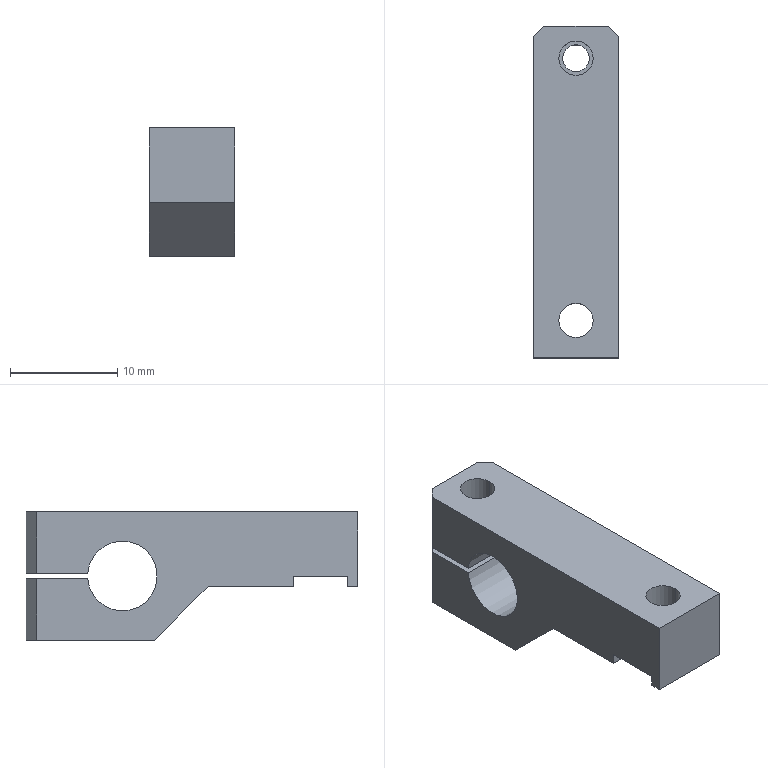Part | SolidWorks | features ICE 4, HoleWzd 3, Chamfer 2, Extrusion 1 | 1 solid | 26 faces | box 8 x 31 x 12 mm | volume 1853 mm3 | plane 19 | cylinder 7 | commonest cylinder face diameters 3.2 x4 2.5 x2 6.5 x1
STEP:
#1=CARTESIAN_POINT('',(-1.6,-12.,0.));
#2=VERTEX_POINT('',#1);
#3=CARTESIAN_POINT('',(1.6,-12.,0.));
#4=VERTEX_POINT('',#3);
#5=CARTESIAN_POINT('',(0.,-12.,0.));
#6=DIRECTION('',(0.,0.,1.));
#7=DIRECTION('',(1.,0.,0.));
#8=AXIS2_PLACEMENT_3D('',#5,#6,#7);
#9=CIRCLE('',#8,1.6);
#10=EDGE_CURVE('',#2,#4,#9,.T.);
#11=ORIENTED_EDGE('',*,*,#10,.F.);
#12=CARTESIAN_POINT('',(-1.6,-12.,6.));
#13=VERTEX_POINT('',#12);
#14=CARTESIAN_POINT('',(-1.6,-12.,6.));
#15=DIRECTION('',(0.,0.,1.));
#16=VECTOR('',#15,1000.);
#17=LINE('',#14,#16);
#18=EDGE_CURVE('',#2,#13,#17,.T.);
#19=ORIENTED_EDGE('',*,*,#18,.T.);
#20=CARTESIAN_POINT('',(1.6,-12.,6.));
#21=VERTEX_POINT('',#20);
#22=CARTESIAN_POINT('',(0.,-12.,6.));
#23=DIRECTION('',(0.,0.,1.));
#24=DIRECTION('',(1.,0.,0.));
#25=AXIS2_PLACEMENT_3D('',#22,#23,#24);
#26=CIRCLE('',#25,1.6);
#27=EDGE_CURVE('',#13,#21,#26,.T.);
#28=ORIENTED_EDGE('',*,*,#27,.T.);
#29=CARTESIAN_POINT('',(1.6,-12.,6.));
#30=DIRECTION('',(0.,0.,1.));
#31=VECTOR('',#30,1000.);
#32=LINE('',#29,#31);
#33=EDGE_CURVE('',#4,#21,#32,.T.);
#34=ORIENTED_EDGE('',*,*,#33,.F.);
#35=EDGE_LOOP('',(#11,#19,#28,#34));
#36=FACE_OUTER_BOUND('',#35,.T.);
#37=CARTESIAN_POINT('',(0.,-12.,6.));
#38=DIRECTION('',(0.,0.,1.));
#39=DIRECTION('',(1.,0.,0.));
#40=AXIS2_PLACEMENT_3D('',#37,#38,#39);
#41=CYLINDRICAL_SURFACE('',#40,1.6);
#42=ADVANCED_FACE('',(#36),#41,.F.);
#43=CARTESIAN_POINT('',(1.6,12.5,0.25));
#44=VERTEX_POINT('',#43);
#45=CARTESIAN_POINT('',(-1.6,12.5,0.25));
#46=VERTEX_POINT('',#45);
#47=CARTESIAN_POINT('',(0.,12.5,0.25));
#48=DIRECTION('',(0.,0.,-1.));
#49=DIRECTION('',(0.,-1.,0.));
#50=AXIS2_PLACEMENT_3D('',#47,#48,#49);
#51=CIRCLE('',#50,1.6);
#52=EDGE_CURVE('',#44,#46,#51,.T.);
#53=ORIENTED_EDGE('',*,*,#52,.T.);
#54=CARTESIAN_POINT('',(-1.6,12.5,6.));
#55=VERTEX_POINT('',#54);
#56=CARTESIAN_POINT('',(-1.6,12.5,6.));
#57=DIRECTION('',(0.,0.,1.));
#58=VECTOR('',#57,1000.);
#59=LINE('',#56,#58);
#60=EDGE_CURVE('',#46,#55,#59,.T.);
#61=ORIENTED_EDGE('',*,*,#60,.T.);
#62=CARTESIAN_POINT('',(1.6,12.5,6.));
#63=VERTEX_POINT('',#62);
#64=CARTESIAN_POINT('',(0.,12.5,6.));
#65=DIRECTION('',(0.,0.,1.));
#66=DIRECTION('',(1.,0.,0.));
#67=AXIS2_PLACEMENT_3D('',#64,#65,#66);
#68=CIRCLE('',#67,1.6);
#69=EDGE_CURVE('',#55,#63,#68,.T.);
#70=ORIENTED_EDGE('',*,*,#69,.T.);
#71=CARTESIAN_POINT('',(1.6,12.5,6.));
#72=DIRECTION('',(0.,0.,1.));
#73=VECTOR('',#72,1000.);
#74=LINE('',#71,#73);
#75=EDGE_CURVE('',#44,#63,#74,.T.);
#76=ORIENTED_EDGE('',*,*,#75,.F.);
#77=EDGE_LOOP('',(#53,#61,#70,#76));
#78=FACE_OUTER_BOUND('',#77,.T.);
#79=CARTESIAN_POINT('',(0.,12.5,6.));
#80=DIRECTION('',(0.,0.,1.));
#81=DIRECTION('',(1.,0.,0.));
#82=AXIS2_PLACEMENT_3D('',#79,#80,#81);
#83=CYLINDRICAL_SURFACE('',#82,1.6);
#84=ADVANCED_FACE('',(#78),#83,.F.);
#85=CARTESIAN_POINT('',(1.25,12.5,-0.25));
#86=VERTEX_POINT('',#85);
#87=CARTESIAN_POINT('',(-1.25,12.5,-0.25));
#88=VERTEX_POINT('',#87);
#89=CARTESIAN_POINT('',(0.,12.5,-0.25));
#90=DIRECTION('',(0.,0.,-1.));
#91=DIRECTION('',(0.,1.,0.));
#92=AXIS2_PLACEMENT_3D('',#89,#90,#91);
#93=CIRCLE('',#92,1.25);
#94=EDGE_CURVE('',#86,#88,#93,.T.);
#95=ORIENTED_EDGE('',*,*,#94,.F.);
#96=CARTESIAN_POINT('',(1.25,12.5,-6.));
#97=VERTEX_POINT('',#96);
#98=CARTESIAN_POINT('',(1.25,12.5,-6.));
#99=DIRECTION('',(0.,0.,-1.));
#100=VECTOR('',#99,1000.);
#101=LINE('',#98,#100);
#102=EDGE_CURVE('',#86,#97,#101,.T.);
#103=ORIENTED_EDGE('',*,*,#102,.T.);
#104=CARTESIAN_POINT('',(-1.25,12.5,-6.));
#105=VERTEX_POINT('',#104);
#106=CARTESIAN_POINT('',(0.,12.5,-6.));
#107=DIRECTION('',(0.,0.,-1.));
#108=DIRECTION('',(-1.,0.,0.));
#109=AXIS2_PLACEMENT_3D('',#106,#107,#108);
#110=CIRCLE('',#109,1.25);
#111=EDGE_CURVE('',#97,#105,#110,.T.);
#112=ORIENTED_EDGE('',*,*,#111,.T.);
#113=CARTESIAN_POINT('',(-1.25,12.5,-6.));
#114=DIRECTION('',(0.,0.,-1.));
#115=VECTOR('',#114,1000.);
#116=LINE('',#113,#115);
#117=EDGE_CURVE('',#88,#105,#116,.T.);
#118=ORIENTED_EDGE('',*,*,#117,.F.);
#119=EDGE_LOOP('',(#95,#103,#112,#118));
#120=FACE_OUTER_BOUND('',#119,.T.);
#121=CARTESIAN_POINT('',(0.,12.5,-6.));
#122=DIRECTION('',(0.,0.,-1.));
#123=DIRECTION('',(-1.,0.,0.));
#124=AXIS2_PLACEMENT_3D('',#121,#122,#123);
#125=CYLINDRICAL_SURFACE('',#124,1.25);
#126=ADVANCED_FACE('',(#120),#125,.F.);
#127=CARTESIAN_POINT('',(-3.,15.5,-0.25));
#128=VERTEX_POINT('',#127);
#129=CARTESIAN_POINT('',(3.,15.5,-0.25));
#130=VERTEX_POINT('',#129);
#131=CARTESIAN_POINT('',(-4.,15.5,-0.25));
#132=DIRECTION('',(1.,0.,0.));
#133=VECTOR('',#132,1000.);
#134=LINE('',#131,#133);
#135=EDGE_CURVE('',#128,#130,#134,.T.);
#136=ORIENTED_EDGE('',*,*,#135,.T.);
#137=CARTESIAN_POINT('',(3.,15.5,-6.));
#138=VERTEX_POINT('',#137);
#139=CARTESIAN_POINT('',(3.,15.5,6.));
#140=DIRECTION('',(0.,0.,-1.));
#141=VECTOR('',#140,1000.);
#142=LINE('',#139,#141);
#143=EDGE_CURVE('',#130,#138,#142,.T.);
#144=ORIENTED_EDGE('',*,*,#143,.T.);
#145=CARTESIAN_POINT('',(-3.,15.5,-6.));
#146=VERTEX_POINT('',#145);
#147=CARTESIAN_POINT('',(-4.,15.5,-6.));
#148=DIRECTION('',(-1.,0.,0.));
#149=VECTOR('',#148,1000.);
#150=LINE('',#147,#149);
#151=EDGE_CURVE('',#138,#146,#150,.T.);
#152=ORIENTED_EDGE('',*,*,#151,.T.);
#153=CARTESIAN_POINT('',(-3.,15.5,6.));
#154=DIRECTION('',(0.,0.,1.));
#155=VECTOR('',#154,1000.);
#156=LINE('',#153,#155);
#157=EDGE_CURVE('',#146,#128,#156,.T.);
#158=ORIENTED_EDGE('',*,*,#157,.T.);
#159=EDGE_LOOP('',(#136,#144,#152,#158));
#160=FACE_OUTER_BOUND('',#159,.T.);
#161=CARTESIAN_POINT('',(-4.,15.5,6.));
#162=DIRECTION('',(0.,-1.,0.));
#163=DIRECTION('',(0.,0.,-1.));
#164=AXIS2_PLACEMENT_3D('',#161,#162,#163);
#165=PLANE('',#164);
#166=ADVANCED_FACE('',(#160),#165,.F.);
#167=CARTESIAN_POINT('',(4.,-1.5,-1.));
#168=VERTEX_POINT('',#167);
#169=CARTESIAN_POINT('',(4.,-9.5,-1.));
#170=VERTEX_POINT('',#169);
#171=CARTESIAN_POINT('',(4.,-15.5,-1.));
#172=DIRECTION('',(0.,-1.,0.));
#173=VECTOR('',#172,1000.);
#174=LINE('',#171,#173);
#175=EDGE_CURVE('',#168,#170,#174,.T.);
#176=ORIENTED_EDGE('',*,*,#175,.T.);
#177=CARTESIAN_POINT('',(-4.,-9.5,-1.));
#178=VERTEX_POINT('',#177);
#179=CARTESIAN_POINT('',(-4.,-9.5,-1.));
#180=DIRECTION('',(1.,0.,0.));
#181=VECTOR('',#180,1000.);
#182=LINE('',#179,#181);
#183=EDGE_CURVE('',#178,#170,#182,.T.);
#184=ORIENTED_EDGE('',*,*,#183,.F.);
#185=CARTESIAN_POINT('',(-4.,-1.5,-1.));
#186=VERTEX_POINT('',#185);
#187=CARTESIAN_POINT('',(-4.,-15.5,-1.));
#188=DIRECTION('',(0.,-1.,0.));
#189=VECTOR('',#188,1000.);
#190=LINE('',#187,#189);
#191=EDGE_CURVE('',#186,#178,#190,.T.);
#192=ORIENTED_EDGE('',*,*,#191,.F.);
#193=CARTESIAN_POINT('',(-4.,-1.5,-1.));
#194=DIRECTION('',(1.,0.,0.));
#195=VECTOR('',#194,1000.);
#196=LINE('',#193,#195);
#197=EDGE_CURVE('',#186,#168,#196,.T.);
#198=ORIENTED_EDGE('',*,*,#197,.T.);
#199=EDGE_LOOP('',(#176,#184,#192,#198));
#200=FACE_OUTER_BOUND('',#199,.T.);
#201=CARTESIAN_POINT('',(-4.,-15.5,-1.));
#202=DIRECTION('',(0.,0.,1.));
#203=DIRECTION('',(1.,0.,0.));
#204=AXIS2_PLACEMENT_3D('',#201,#202,#203);
#205=PLANE('',#204);
#206=ADVANCED_FACE('',(#200),#205,.F.);
#207=CARTESIAN_POINT('',(4.,3.5,-6.));
#208=VERTEX_POINT('',#207);
#209=CARTESIAN_POINT('',(4.,14.5,-6.));
#210=VERTEX_POINT('',#209);
#211=CARTESIAN_POINT('',(4.,15.5,-6.));
#212=DIRECTION('',(0.,1.,0.));
#213=VECTOR('',#212,1000.);
#214=LINE('',#211,#213);
#215=EDGE_CURVE('',#208,#210,#214,.T.);
#216=ORIENTED_EDGE('',*,*,#215,.T.);
#217=CARTESIAN_POINT('',(4.,14.5,-0.25));
#218=VERTEX_POINT('',#217);
#219=CARTESIAN_POINT('',(4.,14.5,6.));
#220=DIRECTION('',(0.,0.,1.));
#221=VECTOR('',#220,1000.);
#222=LINE('',#219,#221);
#223=EDGE_CURVE('',#210,#218,#222,.T.);
#224=ORIENTED_EDGE('',*,*,#223,.T.);
#225=CARTESIAN_POINT('',(4.,9.74,-0.25));
#226=VERTEX_POINT('',#225);
#227=CARTESIAN_POINT('',(4.,15.5,-0.25));
#228=DIRECTION('',(0.,1.,0.));
#229=VECTOR('',#228,1000.);
#230=LINE('',#227,#229);
#231=EDGE_CURVE('',#226,#218,#230,.T.);
#232=ORIENTED_EDGE('',*,*,#231,.F.);
#233=CARTESIAN_POINT('',(4.,9.74,0.25));
#234=VERTEX_POINT('',#233);
#235=CARTESIAN_POINT('',(4.,6.5,0.));
#236=DIRECTION('',(1.,0.,0.));
#237=DIRECTION('',(0.,1.,0.));
#238=AXIS2_PLACEMENT_3D('',#235,#236,#237);
#239=CIRCLE('',#238,3.25);
#240=EDGE_CURVE('',#234,#226,#239,.T.);
#241=ORIENTED_EDGE('',*,*,#240,.F.);
#242=CARTESIAN_POINT('',(4.,14.5,0.25));
#243=VERTEX_POINT('',#242);
#244=CARTESIAN_POINT('',(4.,15.5,0.25));
#245=DIRECTION('',(0.,-1.,0.));
#246=VECTOR('',#245,1000.);
#247=LINE('',#244,#246);
#248=EDGE_CURVE('',#243,#234,#247,.T.);
#249=ORIENTED_EDGE('',*,*,#248,.F.);
#250=CARTESIAN_POINT('',(4.,14.5,6.));
#251=VERTEX_POINT('',#250);
#252=CARTESIAN_POINT('',(4.,14.5,6.));
#253=DIRECTION('',(0.,0.,1.));
#254=VECTOR('',#253,1000.);
#255=LINE('',#252,#254);
#256=EDGE_CURVE('',#243,#251,#255,.T.);
#257=ORIENTED_EDGE('',*,*,#256,.T.);
#258=CARTESIAN_POINT('',(4.,-15.5,6.));
#259=VERTEX_POINT('',#258);
#260=CARTESIAN_POINT('',(4.,15.5,6.));
#261=DIRECTION('',(0.,1.,0.));
#262=VECTOR('',#261,1000.);
#263=LINE('',#260,#262);
#264=EDGE_CURVE('',#259,#251,#263,.T.);
#265=ORIENTED_EDGE('',*,*,#264,.F.);
#266=CARTESIAN_POINT('',(4.,-15.5,-1.));
#267=VERTEX_POINT('',#266);
#268=CARTESIAN_POINT('',(4.,-15.5,6.));
#269=DIRECTION('',(0.,0.,-1.));
#270=VECTOR('',#269,1000.);
#271=LINE('',#268,#270);
#272=EDGE_CURVE('',#259,#267,#271,.T.);
#273=ORIENTED_EDGE('',*,*,#272,.T.);
#274=CARTESIAN_POINT('',(4.,-14.5,-1.));
#275=VERTEX_POINT('',#274);
#276=CARTESIAN_POINT('',(4.,-15.5,-1.));
#277=DIRECTION('',(0.,-1.,0.));
#278=VECTOR('',#277,1000.);
#279=LINE('',#276,#278);
#280=EDGE_CURVE('',#275,#267,#279,.T.);
#281=ORIENTED_EDGE('',*,*,#280,.F.);
#282=CARTESIAN_POINT('',(4.,-14.5,0.));
#283=VERTEX_POINT('',#282);
#284=CARTESIAN_POINT('',(4.,-14.5,0.));
#285=DIRECTION('',(0.,0.,-1.));
#286=VECTOR('',#285,1000.);
#287=LINE('',#284,#286);
#288=EDGE_CURVE('',#283,#275,#287,.T.);
#289=ORIENTED_EDGE('',*,*,#288,.F.);
#290=CARTESIAN_POINT('',(4.,-9.5,0.));
#291=VERTEX_POINT('',#290);
#292=CARTESIAN_POINT('',(4.,-14.5,0.));
#293=DIRECTION('',(0.,-1.,0.));
#294=VECTOR('',#293,1000.);
#295=LINE('',#292,#294);
#296=EDGE_CURVE('',#291,#283,#295,.T.);
#297=ORIENTED_EDGE('',*,*,#296,.F.);
#298=CARTESIAN_POINT('',(4.,-9.5,0.));
#299=DIRECTION('',(0.,0.,1.));
#300=VECTOR('',#299,1000.);
#301=LINE('',#298,#300);
#302=EDGE_CURVE('',#170,#291,#301,.T.);
#303=ORIENTED_EDGE('',*,*,#302,.F.);
#304=ORIENTED_EDGE('',*,*,#175,.F.);
#305=CARTESIAN_POINT('',(4.,-1.5,-1.));
#306=DIRECTION('',(0.,0.7071,-0.7071));
#307=VECTOR('',#306,1000.);
#308=LINE('',#305,#307);
#309=EDGE_CURVE('',#168,#208,#308,.T.);
#310=ORIENTED_EDGE('',*,*,#309,.T.);
#311=EDGE_LOOP('',(#216,#224,#232,#241,#249,#257,#265,#273,#281,#289,#297,#303,#304,#310));
#312=FACE_OUTER_BOUND('',#311,.T.);
#313=CARTESIAN_POINT('',(4.,15.5,6.));
#314=DIRECTION('',(-1.,0.,0.));
#315=DIRECTION('',(0.,-1.,0.));
#316=AXIS2_PLACEMENT_3D('',#313,#314,#315);
#317=PLANE('',#316);
#318=ADVANCED_FACE('',(#312),#317,.F.);
#319=CARTESIAN_POINT('',(-3.,15.5,0.25));
#320=VERTEX_POINT('',#319);
#321=CARTESIAN_POINT('',(3.,15.5,0.25));
#322=VERTEX_POINT('',#321);
#323=CARTESIAN_POINT('',(-4.,15.5,0.25));
#324=DIRECTION('',(1.,0.,0.));
#325=VECTOR('',#324,1000.);
#326=LINE('',#323,#325);
#327=EDGE_CURVE('',#320,#322,#326,.T.);
#328=ORIENTED_EDGE('',*,*,#327,.F.);
#329=CARTESIAN_POINT('',(-3.,15.5,6.));
#330=VERTEX_POINT('',#329);
#331=CARTESIAN_POINT('',(-3.,15.5,6.));
#332=DIRECTION('',(0.,0.,1.));
#333=VECTOR('',#332,1000.);
#334=LINE('',#331,#333);
#335=EDGE_CURVE('',#320,#330,#334,.T.);
#336=ORIENTED_EDGE('',*,*,#335,.T.);
#337=CARTESIAN_POINT('',(3.,15.5,6.));
#338=VERTEX_POINT('',#337);
#339=CARTESIAN_POINT('',(-4.,15.5,6.));
#340=DIRECTION('',(-1.,0.,0.));
#341=VECTOR('',#340,1000.);
#342=LINE('',#339,#341);
#343=EDGE_CURVE('',#338,#330,#342,.T.);
#344=ORIENTED_EDGE('',*,*,#343,.F.);
#345=CARTESIAN_POINT('',(3.,15.5,6.));
#346=DIRECTION('',(0.,0.,-1.));
#347=VECTOR('',#346,1000.);
#348=LINE('',#345,#347);
#349=EDGE_CURVE('',#338,#322,#348,.T.);
#350=ORIENTED_EDGE('',*,*,#349,.T.);
#351=EDGE_LOOP('',(#328,#336,#344,#350));
#352=FACE_OUTER_BOUND('',#351,.T.);
#353=CARTESIAN_POINT('',(-4.,15.5,6.));
#354=DIRECTION('',(0.,-1.,0.));
#355=DIRECTION('',(0.,0.,-1.));
#356=AXIS2_PLACEMENT_3D('',#353,#354,#355);
#357=PLANE('',#356);
#358=ADVANCED_FACE('',(#352),#357,.F.);
#359=CARTESIAN_POINT('',(-4.,9.74,-0.25));
#360=VERTEX_POINT('',#359);
#361=CARTESIAN_POINT('',(-4.,14.5,-0.25));
#362=VERTEX_POINT('',#361);
#363=CARTESIAN_POINT('',(-4.,15.5,-0.25));
#364=DIRECTION('',(0.,1.,0.));
#365=VECTOR('',#364,1000.);
#366=LINE('',#363,#365);
#367=EDGE_CURVE('',#360,#362,#366,.T.);
#368=ORIENTED_EDGE('',*,*,#367,.T.);
#369=CARTESIAN_POINT('',(-4.,14.5,-6.));
#370=VERTEX_POINT('',#369);
#371=CARTESIAN_POINT('',(-4.,14.5,6.));
#372=DIRECTION('',(0.,0.,-1.));
#373=VECTOR('',#372,1000.);
#374=LINE('',#371,#373);
#375=EDGE_CURVE('',#362,#370,#374,.T.);
#376=ORIENTED_EDGE('',*,*,#375,.T.);
#377=CARTESIAN_POINT('',(-4.,3.5,-6.));
#378=VERTEX_POINT('',#377);
#379=CARTESIAN_POINT('',(-4.,15.5,-6.));
#380=DIRECTION('',(0.,-1.,0.));
#381=VECTOR('',#380,1000.);
#382=LINE('',#379,#381);
#383=EDGE_CURVE('',#370,#378,#382,.T.);
#384=ORIENTED_EDGE('',*,*,#383,.T.);
#385=CARTESIAN_POINT('',(-4.,-1.5,-1.));
#386=DIRECTION('',(0.,-0.7071,0.7071));
#387=VECTOR('',#386,1000.);
#388=LINE('',#385,#387);
#389=EDGE_CURVE('',#378,#186,#388,.T.);
#390=ORIENTED_EDGE('',*,*,#389,.T.);
#391=ORIENTED_EDGE('',*,*,#191,.T.);
#392=CARTESIAN_POINT('',(-4.,-9.5,0.));
#393=VERTEX_POINT('',#392);
#394=CARTESIAN_POINT('',(-4.,-9.5,0.));
#395=DIRECTION('',(0.,0.,1.));
#396=VECTOR('',#395,1000.);
#397=LINE('',#394,#396);
#398=EDGE_CURVE('',#178,#393,#397,.T.);
#399=ORIENTED_EDGE('',*,*,#398,.T.);
#400=CARTESIAN_POINT('',(-4.,-14.5,0.));
#401=VERTEX_POINT('',#400);
#402=CARTESIAN_POINT('',(-4.,-14.5,0.));
#403=DIRECTION('',(0.,-1.,0.));
#404=VECTOR('',#403,1000.);
#405=LINE('',#402,#404);
#406=EDGE_CURVE('',#393,#401,#405,.T.);
#407=ORIENTED_EDGE('',*,*,#406,.T.);
#408=CARTESIAN_POINT('',(-4.,-14.5,-1.));
#409=VERTEX_POINT('',#408);
#410=CARTESIAN_POINT('',(-4.,-14.5,0.));
#411=DIRECTION('',(0.,0.,-1.));
#412=VECTOR('',#411,1000.);
#413=LINE('',#410,#412);
#414=EDGE_CURVE('',#401,#409,#413,.T.);
#415=ORIENTED_EDGE('',*,*,#414,.T.);
#416=CARTESIAN_POINT('',(-4.,-15.5,-1.));
#417=VERTEX_POINT('',#416);
#418=CARTESIAN_POINT('',(-4.,-15.5,-1.));
#419=DIRECTION('',(0.,-1.,0.));
#420=VECTOR('',#419,1000.);
#421=LINE('',#418,#420);
#422=EDGE_CURVE('',#409,#417,#421,.T.);
#423=ORIENTED_EDGE('',*,*,#422,.T.);
#424=CARTESIAN_POINT('',(-4.,-15.5,6.));
#425=VERTEX_POINT('',#424);
#426=CARTESIAN_POINT('',(-4.,-15.5,6.));
#427=DIRECTION('',(0.,0.,-1.));
#428=VECTOR('',#427,1000.);
#429=LINE('',#426,#428);
#430=EDGE_CURVE('',#425,#417,#429,.T.);
#431=ORIENTED_EDGE('',*,*,#430,.F.);
#432=CARTESIAN_POINT('',(-4.,14.5,6.));
#433=VERTEX_POINT('',#432);
#434=CARTESIAN_POINT('',(-4.,15.5,6.));
#435=DIRECTION('',(0.,-1.,0.));
#436=VECTOR('',#435,1000.);
#437=LINE('',#434,#436);
#438=EDGE_CURVE('',#433,#425,#437,.T.);
#439=ORIENTED_EDGE('',*,*,#438,.F.);
#440=CARTESIAN_POINT('',(-4.,14.5,0.25));
#441=VERTEX_POINT('',#440);
#442=CARTESIAN_POINT('',(-4.,14.5,6.));
#443=DIRECTION('',(0.,0.,-1.));
#444=VECTOR('',#443,1000.);
#445=LINE('',#442,#444);
#446=EDGE_CURVE('',#433,#441,#445,.T.);
#447=ORIENTED_EDGE('',*,*,#446,.T.);
#448=CARTESIAN_POINT('',(-4.,9.74,0.25));
#449=VERTEX_POINT('',#448);
#450=CARTESIAN_POINT('',(-4.,15.5,0.25));
#451=DIRECTION('',(0.,-1.,0.));
#452=VECTOR('',#451,1000.);
#453=LINE('',#450,#452);
#454=EDGE_CURVE('',#441,#449,#453,.T.);
#455=ORIENTED_EDGE('',*,*,#454,.T.);
#456=CARTESIAN_POINT('',(-4.,6.5,0.));
#457=DIRECTION('',(1.,0.,0.));
#458=DIRECTION('',(0.,1.,0.));
#459=AXIS2_PLACEMENT_3D('',#456,#457,#458);
#460=CIRCLE('',#459,3.25);
#461=EDGE_CURVE('',#449,#360,#460,.T.);
#462=ORIENTED_EDGE('',*,*,#461,.T.);
#463=EDGE_LOOP('',(#368,#376,#384,#390,#391,#399,#407,#415,#423,#431,#439,#447,#455,#462));
#464=FACE_OUTER_BOUND('',#463,.T.);
#465=CARTESIAN_POINT('',(-4.,15.5,6.));
#466=DIRECTION('',(1.,0.,0.));
#467=DIRECTION('',(0.,1.,0.));
#468=AXIS2_PLACEMENT_3D('',#465,#466,#467);
#469=PLANE('',#468);
#470=ADVANCED_FACE('',(#464),#469,.F.);
#471=ORIENTED_EDGE('',*,*,#430,.T.);
#472=CARTESIAN_POINT('',(-4.,-15.5,-1.));
#473=DIRECTION('',(1.,0.,0.));
#474=VECTOR('',#473,1000.);
#475=LINE('',#472,#474);
#476=EDGE_CURVE('',#417,#267,#475,.T.);
#477=ORIENTED_EDGE('',*,*,#476,.T.);
#478=ORIENTED_EDGE('',*,*,#272,.F.);
#479=CARTESIAN_POINT('',(-4.,-15.5,6.));
#480=DIRECTION('',(1.,0.,0.));
#481=VECTOR('',#480,1000.);
#482=LINE('',#479,#481);
#483=EDGE_CURVE('',#425,#259,#482,.T.);
#484=ORIENTED_EDGE('',*,*,#483,.F.);
#485=EDGE_LOOP('',(#471,#477,#478,#484));
#486=FACE_OUTER_BOUND('',#485,.T.);
#487=CARTESIAN_POINT('',(-4.,-15.5,6.));
#488=DIRECTION('',(0.,1.,0.));
#489=DIRECTION('',(0.,0.,1.));
#490=AXIS2_PLACEMENT_3D('',#487,#488,#489);
#491=PLANE('',#490);
#492=ADVANCED_FACE('',(#486),#491,.F.);
#493=CARTESIAN_POINT('',(0.,-12.,6.));
#494=DIRECTION('',(0.,0.,1.));
#495=DIRECTION('',(1.,0.,0.));
#496=AXIS2_PLACEMENT_3D('',#493,#494,#495);
#497=CIRCLE('',#496,1.6);
#498=EDGE_CURVE('',#21,#13,#497,.T.);
#499=ORIENTED_EDGE('',*,*,#498,.F.);
#500=ORIENTED_EDGE('',*,*,#27,.F.);
#501=EDGE_LOOP('',(#499,#500));
#502=FACE_BOUND('',#501,.T.);
#503=CARTESIAN_POINT('',(0.,12.5,6.));
#504=DIRECTION('',(0.,0.,1.));
#505=DIRECTION('',(1.,0.,0.));
#506=AXIS2_PLACEMENT_3D('',#503,#504,#505);
#507=CIRCLE('',#506,1.6);
#508=EDGE_CURVE('',#63,#55,#507,.T.);
#509=ORIENTED_EDGE('',*,*,#508,.F.);
#510=ORIENTED_EDGE('',*,*,#69,.F.);
#511=EDGE_LOOP('',(#509,#510));
#512=FACE_BOUND('',#511,.T.);
#513=ORIENTED_EDGE('',*,*,#343,.T.);
#514=CARTESIAN_POINT('',(-9.25,9.25,6.));
#515=DIRECTION('',(-0.7071,-0.7071,0.));
#516=VECTOR('',#515,1000.);
#517=LINE('',#514,#516);
#518=EDGE_CURVE('',#330,#433,#517,.T.);
#519=ORIENTED_EDGE('',*,*,#518,.T.);
#520=ORIENTED_EDGE('',*,*,#438,.T.);
#521=ORIENTED_EDGE('',*,*,#483,.T.);
#522=ORIENTED_EDGE('',*,*,#264,.T.);
#523=CARTESIAN_POINT('',(9.25,9.25,6.));
#524=DIRECTION('',(-0.7071,0.7071,0.));
#525=VECTOR('',#524,1000.);
#526=LINE('',#523,#525);
#527=EDGE_CURVE('',#251,#338,#526,.T.);
#528=ORIENTED_EDGE('',*,*,#527,.T.);
#529=EDGE_LOOP('',(#513,#519,#520,#521,#522,#528));
#530=FACE_OUTER_BOUND('',#529,.T.);
#531=CARTESIAN_POINT('',(0.,0.,6.));
#532=DIRECTION('',(0.,0.,1.));
#533=DIRECTION('',(1.,0.,0.));
#534=AXIS2_PLACEMENT_3D('',#531,#532,#533);
#535=PLANE('',#534);
#536=ADVANCED_FACE('',(#502,#512,#530),#535,.T.);
#537=CARTESIAN_POINT('',(0.,12.5,-6.));
#538=DIRECTION('',(0.,0.,-1.));
#539=DIRECTION('',(-1.,0.,0.));
#540=AXIS2_PLACEMENT_3D('',#537,#538,#539);
#541=CIRCLE('',#540,1.25);
#542=EDGE_CURVE('',#105,#97,#541,.T.);
#543=ORIENTED_EDGE('',*,*,#542,.F.);
#544=ORIENTED_EDGE('',*,*,#111,.F.);
#545=EDGE_LOOP('',(#543,#544));
#546=FACE_BOUND('',#545,.T.);
#547=ORIENTED_EDGE('',*,*,#151,.F.);
#548=CARTESIAN_POINT('',(3.,15.5,-6.));
#549=DIRECTION('',(0.7071,-0.7071,0.));
#550=VECTOR('',#549,1000.);
#551=LINE('',#548,#550);
#552=EDGE_CURVE('',#138,#210,#551,.T.);
#553=ORIENTED_EDGE('',*,*,#552,.T.);
#554=ORIENTED_EDGE('',*,*,#215,.F.);
#555=CARTESIAN_POINT('',(0.,3.5,-6.));
#556=DIRECTION('',(-1.,0.,0.));
#557=VECTOR('',#556,1000.);
#558=LINE('',#555,#557);
#559=EDGE_CURVE('',#208,#378,#558,.T.);
#560=ORIENTED_EDGE('',*,*,#559,.T.);
#561=ORIENTED_EDGE('',*,*,#383,.F.);
#562=CARTESIAN_POINT('',(-4.,14.5,-6.));
#563=DIRECTION('',(0.7071,0.7071,0.));
#564=VECTOR('',#563,1000.);
#565=LINE('',#562,#564);
#566=EDGE_CURVE('',#370,#146,#565,.T.);
#567=ORIENTED_EDGE('',*,*,#566,.T.);
#568=EDGE_LOOP('',(#547,#553,#554,#560,#561,#567));
#569=FACE_OUTER_BOUND('',#568,.T.);
#570=CARTESIAN_POINT('',(0.,0.,-6.));
#571=DIRECTION('',(0.,0.,1.));
#572=DIRECTION('',(1.,0.,0.));
#573=AXIS2_PLACEMENT_3D('',#570,#571,#572);
#574=PLANE('',#573);
#575=ADVANCED_FACE('',(#546,#569),#574,.F.);
#576=ORIENTED_EDGE('',*,*,#422,.F.);
#577=CARTESIAN_POINT('',(-4.,-14.5,-1.));
#578=DIRECTION('',(1.,0.,0.));
#579=VECTOR('',#578,1000.);
#580=LINE('',#577,#579);
#581=EDGE_CURVE('',#409,#275,#580,.T.);
#582=ORIENTED_EDGE('',*,*,#581,.T.);
#583=ORIENTED_EDGE('',*,*,#280,.T.);
#584=ORIENTED_EDGE('',*,*,#476,.F.);
#585=EDGE_LOOP('',(#576,#582,#583,#584));
#586=FACE_OUTER_BOUND('',#585,.T.);
#587=CARTESIAN_POINT('',(-4.,-15.5,-1.));
#588=DIRECTION('',(0.,0.,1.));
#589=DIRECTION('',(1.,0.,0.));
#590=AXIS2_PLACEMENT_3D('',#587,#588,#589);
#591=PLANE('',#590);
#592=ADVANCED_FACE('',(#586),#591,.F.);
#593=CARTESIAN_POINT('',(0.,-12.,0.));
#594=DIRECTION('',(0.,0.,1.));
#595=DIRECTION('',(1.,0.,0.));
#596=AXIS2_PLACEMENT_3D('',#593,#594,#595);
#597=CIRCLE('',#596,1.6);
#598=EDGE_CURVE('',#4,#2,#597,.T.);
#599=ORIENTED_EDGE('',*,*,#598,.T.);
#600=ORIENTED_EDGE('',*,*,#10,.T.);
#601=EDGE_LOOP('',(#599,#600));
#602=FACE_BOUND('',#601,.T.);
#603=ORIENTED_EDGE('',*,*,#296,.T.);
#604=CARTESIAN_POINT('',(-4.,-14.5,0.));
#605=DIRECTION('',(1.,0.,0.));
#606=VECTOR('',#605,1000.);
#607=LINE('',#604,#606);
#608=EDGE_CURVE('',#401,#283,#607,.T.);
#609=ORIENTED_EDGE('',*,*,#608,.F.);
#610=ORIENTED_EDGE('',*,*,#406,.F.);
#611=CARTESIAN_POINT('',(-4.,-9.5,0.));
#612=DIRECTION('',(1.,0.,0.));
#613=VECTOR('',#612,1000.);
#614=LINE('',#611,#613);
#615=EDGE_CURVE('',#393,#291,#614,.T.);
#616=ORIENTED_EDGE('',*,*,#615,.T.);
#617=EDGE_LOOP('',(#603,#609,#610,#616));
#618=FACE_OUTER_BOUND('',#617,.T.);
#619=CARTESIAN_POINT('',(-4.,-14.5,0.));
#620=DIRECTION('',(0.,0.,1.));
#621=DIRECTION('',(1.,0.,0.));
#622=AXIS2_PLACEMENT_3D('',#619,#620,#621);
#623=PLANE('',#622);
#624=ADVANCED_FACE('',(#602,#618),#623,.F.);
#625=ORIENTED_EDGE('',*,*,#302,.T.);
#626=ORIENTED_EDGE('',*,*,#615,.F.);
#627=ORIENTED_EDGE('',*,*,#398,.F.);
#628=ORIENTED_EDGE('',*,*,#183,.T.);
#629=EDGE_LOOP('',(#625,#626,#627,#628));
#630=FACE_OUTER_BOUND('',#629,.T.);
#631=CARTESIAN_POINT('',(-4.,-9.5,0.));
#632=DIRECTION('',(0.,1.,0.));
#633=DIRECTION('',(-1.,0.,0.));
#634=AXIS2_PLACEMENT_3D('',#631,#632,#633);
#635=PLANE('',#634);
#636=ADVANCED_FACE('',(#630),#635,.F.);
#637=ORIENTED_EDGE('',*,*,#288,.T.);
#638=ORIENTED_EDGE('',*,*,#581,.F.);
#639=ORIENTED_EDGE('',*,*,#414,.F.);
#640=ORIENTED_EDGE('',*,*,#608,.T.);
#641=EDGE_LOOP('',(#637,#638,#639,#640));
#642=FACE_OUTER_BOUND('',#641,.T.);
#643=CARTESIAN_POINT('',(-4.,-14.5,0.));
#644=DIRECTION('',(0.,-1.,0.));
#645=DIRECTION('',(1.,0.,0.));
#646=AXIS2_PLACEMENT_3D('',#643,#644,#645);
#647=PLANE('',#646);
#648=ADVANCED_FACE('',(#642),#647,.F.);
#649=ORIENTED_EDGE('',*,*,#240,.T.);
#650=CARTESIAN_POINT('',(-4.,9.74,-0.25));
#651=DIRECTION('',(-1.,0.,0.));
#652=VECTOR('',#651,1000.);
#653=LINE('',#650,#652);
#654=EDGE_CURVE('',#226,#360,#653,.T.);
#655=ORIENTED_EDGE('',*,*,#654,.T.);
#656=ORIENTED_EDGE('',*,*,#461,.F.);
#657=CARTESIAN_POINT('',(-4.,9.74,0.25));
#658=DIRECTION('',(1.,0.,0.));
#659=VECTOR('',#658,1000.);
#660=LINE('',#657,#659);
#661=EDGE_CURVE('',#449,#234,#660,.T.);
#662=ORIENTED_EDGE('',*,*,#661,.T.);
#663=EDGE_LOOP('',(#649,#655,#656,#662));
#664=FACE_OUTER_BOUND('',#663,.T.);
#665=CARTESIAN_POINT('',(-4.,6.5,0.));
#666=DIRECTION('',(1.,0.,0.));
#667=DIRECTION('',(0.,1.,0.));
#668=AXIS2_PLACEMENT_3D('',#665,#666,#667);
#669=CYLINDRICAL_SURFACE('',#668,3.25);
#670=ADVANCED_FACE('',(#664),#669,.F.);
#671=ORIENTED_EDGE('',*,*,#389,.F.);
#672=ORIENTED_EDGE('',*,*,#559,.F.);
#673=ORIENTED_EDGE('',*,*,#309,.F.);
#674=ORIENTED_EDGE('',*,*,#197,.F.);
#675=EDGE_LOOP('',(#671,#672,#673,#674));
#676=FACE_OUTER_BOUND('',#675,.T.);
#677=CARTESIAN_POINT('',(-4.,-1.5,-1.));
#678=DIRECTION('',(0.,0.7071,0.7071));
#679=DIRECTION('',(1.,0.,0.));
#680=AXIS2_PLACEMENT_3D('',#677,#678,#679);
#681=PLANE('',#680);
#682=ADVANCED_FACE('',(#676),#681,.F.);
#683=ORIENTED_EDGE('',*,*,#52,.F.);
#684=CARTESIAN_POINT('',(0.,12.5,0.25));
#685=DIRECTION('',(0.,0.,-1.));
#686=DIRECTION('',(0.,-1.,0.));
#687=AXIS2_PLACEMENT_3D('',#684,#685,#686);
#688=CIRCLE('',#687,1.6);
#689=EDGE_CURVE('',#46,#44,#688,.T.);
#690=ORIENTED_EDGE('',*,*,#689,.F.);
#691=EDGE_LOOP('',(#683,#690));
#692=FACE_BOUND('',#691,.T.);
#693=ORIENTED_EDGE('',*,*,#454,.F.);
#694=CARTESIAN_POINT('',(-4.,14.5,0.25));
#695=DIRECTION('',(0.7071,0.7071,0.));
#696=VECTOR('',#695,1000.);
#697=LINE('',#694,#696);
#698=EDGE_CURVE('',#441,#320,#697,.T.);
#699=ORIENTED_EDGE('',*,*,#698,.T.);
#700=ORIENTED_EDGE('',*,*,#327,.T.);
#701=CARTESIAN_POINT('',(3.,15.5,0.25));
#702=DIRECTION('',(0.7071,-0.7071,0.));
#703=VECTOR('',#702,1000.);
#704=LINE('',#701,#703);
#705=EDGE_CURVE('',#322,#243,#704,.T.);
#706=ORIENTED_EDGE('',*,*,#705,.T.);
#707=ORIENTED_EDGE('',*,*,#248,.T.);
#708=ORIENTED_EDGE('',*,*,#661,.F.);
#709=EDGE_LOOP('',(#693,#699,#700,#706,#707,#708));
#710=FACE_OUTER_BOUND('',#709,.T.);
#711=CARTESIAN_POINT('',(-4.,15.5,0.25));
#712=DIRECTION('',(0.,0.,1.));
#713=DIRECTION('',(0.,-1.,0.));
#714=AXIS2_PLACEMENT_3D('',#711,#712,#713);
#715=PLANE('',#714);
#716=ADVANCED_FACE('',(#692,#710),#715,.F.);
#717=CARTESIAN_POINT('',(0.,12.5,-0.25));
#718=DIRECTION('',(0.,0.,-1.));
#719=DIRECTION('',(0.,1.,0.));
#720=AXIS2_PLACEMENT_3D('',#717,#718,#719);
#721=CIRCLE('',#720,1.25);
#722=EDGE_CURVE('',#88,#86,#721,.T.);
#723=ORIENTED_EDGE('',*,*,#722,.T.);
#724=ORIENTED_EDGE('',*,*,#94,.T.);
#725=EDGE_LOOP('',(#723,#724));
#726=FACE_BOUND('',#725,.T.);
#727=ORIENTED_EDGE('',*,*,#231,.T.);
#728=CARTESIAN_POINT('',(3.,15.5,-0.25));
#729=DIRECTION('',(-0.7071,0.7071,0.));
#730=VECTOR('',#729,1000.);
#731=LINE('',#728,#730);
#732=EDGE_CURVE('',#218,#130,#731,.T.);
#733=ORIENTED_EDGE('',*,*,#732,.T.);
#734=ORIENTED_EDGE('',*,*,#135,.F.);
#735=CARTESIAN_POINT('',(-4.,14.5,-0.25));
#736=DIRECTION('',(-0.7071,-0.7071,0.));
#737=VECTOR('',#736,1000.);
#738=LINE('',#735,#737);
#739=EDGE_CURVE('',#128,#362,#738,.T.);
#740=ORIENTED_EDGE('',*,*,#739,.T.);
#741=ORIENTED_EDGE('',*,*,#367,.F.);
#742=ORIENTED_EDGE('',*,*,#654,.F.);
#743=EDGE_LOOP('',(#727,#733,#734,#740,#741,#742));
#744=FACE_OUTER_BOUND('',#743,.T.);
#745=CARTESIAN_POINT('',(-4.,15.5,-0.25));
#746=DIRECTION('',(0.,0.,-1.));
#747=DIRECTION('',(0.,1.,0.));
#748=AXIS2_PLACEMENT_3D('',#745,#746,#747);
#749=PLANE('',#748);
#750=ADVANCED_FACE('',(#726,#744),#749,.F.);
#751=ORIENTED_EDGE('',*,*,#102,.F.);
#752=ORIENTED_EDGE('',*,*,#722,.F.);
#753=ORIENTED_EDGE('',*,*,#117,.T.);
#754=ORIENTED_EDGE('',*,*,#542,.T.);
#755=EDGE_LOOP('',(#751,#752,#753,#754));
#756=FACE_OUTER_BOUND('',#755,.T.);
#757=CARTESIAN_POINT('',(0.,12.5,-6.));
#758=DIRECTION('',(0.,0.,-1.));
#759=DIRECTION('',(-1.,0.,0.));
#760=AXIS2_PLACEMENT_3D('',#757,#758,#759);
#761=CYLINDRICAL_SURFACE('',#760,1.25);
#762=ADVANCED_FACE('',(#756),#761,.F.);
#763=ORIENTED_EDGE('',*,*,#60,.F.);
#764=ORIENTED_EDGE('',*,*,#689,.T.);
#765=ORIENTED_EDGE('',*,*,#75,.T.);
#766=ORIENTED_EDGE('',*,*,#508,.T.);
#767=EDGE_LOOP('',(#763,#764,#765,#766));
#768=FACE_OUTER_BOUND('',#767,.T.);
#769=CARTESIAN_POINT('',(0.,12.5,6.));
#770=DIRECTION('',(0.,0.,1.));
#771=DIRECTION('',(1.,0.,0.));
#772=AXIS2_PLACEMENT_3D('',#769,#770,#771);
#773=CYLINDRICAL_SURFACE('',#772,1.6);
#774=ADVANCED_FACE('',(#768),#773,.F.);
#775=ORIENTED_EDGE('',*,*,#732,.F.);
#776=ORIENTED_EDGE('',*,*,#223,.F.);
#777=ORIENTED_EDGE('',*,*,#552,.F.);
#778=ORIENTED_EDGE('',*,*,#143,.F.);
#779=EDGE_LOOP('',(#775,#776,#777,#778));
#780=FACE_OUTER_BOUND('',#779,.T.);
#781=CARTESIAN_POINT('',(3.,15.5,6.));
#782=DIRECTION('',(-0.7071,-0.7071,0.));
#783=DIRECTION('',(0.,0.,-1.));
#784=AXIS2_PLACEMENT_3D('',#781,#782,#783);
#785=PLANE('',#784);
#786=ADVANCED_FACE('',(#780),#785,.F.);
#787=ORIENTED_EDGE('',*,*,#739,.F.);
#788=ORIENTED_EDGE('',*,*,#157,.F.);
#789=ORIENTED_EDGE('',*,*,#566,.F.);
#790=ORIENTED_EDGE('',*,*,#375,.F.);
#791=EDGE_LOOP('',(#787,#788,#789,#790));
#792=FACE_OUTER_BOUND('',#791,.T.);
#793=CARTESIAN_POINT('',(-4.,14.5,6.));
#794=DIRECTION('',(0.7071,-0.7071,0.));
#795=DIRECTION('',(0.,0.,-1.));
#796=AXIS2_PLACEMENT_3D('',#793,#794,#795);
#797=PLANE('',#796);
#798=ADVANCED_FACE('',(#792),#797,.F.);
#799=ORIENTED_EDGE('',*,*,#518,.F.);
#800=ORIENTED_EDGE('',*,*,#335,.F.);
#801=ORIENTED_EDGE('',*,*,#698,.F.);
#802=ORIENTED_EDGE('',*,*,#446,.F.);
#803=EDGE_LOOP('',(#799,#800,#801,#802));
#804=FACE_OUTER_BOUND('',#803,.T.);
#805=CARTESIAN_POINT('',(-4.,14.5,6.));
#806=DIRECTION('',(0.7071,-0.7071,0.));
#807=DIRECTION('',(0.,0.,-1.));
#808=AXIS2_PLACEMENT_3D('',#805,#806,#807);
#809=PLANE('',#808);
#810=ADVANCED_FACE('',(#804),#809,.F.);
#811=ORIENTED_EDGE('',*,*,#527,.F.);
#812=ORIENTED_EDGE('',*,*,#256,.F.);
#813=ORIENTED_EDGE('',*,*,#705,.F.);
#814=ORIENTED_EDGE('',*,*,#349,.F.);
#815=EDGE_LOOP('',(#811,#812,#813,#814));
#816=FACE_OUTER_BOUND('',#815,.T.);
#817=CARTESIAN_POINT('',(3.,15.5,6.));
#818=DIRECTION('',(-0.7071,-0.7071,0.));
#819=DIRECTION('',(0.,0.,-1.));
#820=AXIS2_PLACEMENT_3D('',#817,#818,#819);
#821=PLANE('',#820);
#822=ADVANCED_FACE('',(#816),#821,.F.);
#823=ORIENTED_EDGE('',*,*,#18,.F.);
#824=ORIENTED_EDGE('',*,*,#598,.F.);
#825=ORIENTED_EDGE('',*,*,#33,.T.);
#826=ORIENTED_EDGE('',*,*,#498,.T.);
#827=EDGE_LOOP('',(#823,#824,#825,#826));
#828=FACE_OUTER_BOUND('',#827,.T.);
#829=CARTESIAN_POINT('',(0.,-12.,6.));
#830=DIRECTION('',(0.,0.,1.));
#831=DIRECTION('',(1.,0.,0.));
#832=AXIS2_PLACEMENT_3D('',#829,#830,#831);
#833=CYLINDRICAL_SURFACE('',#832,1.6);
#834=ADVANCED_FACE('',(#828),#833,.F.);
#835=CLOSED_SHELL('',(#42,#84,#126,#166,#206,#318,#358,#470,#492,#536,#575,#592,#624,#636,#648,#670,#682,#716,#750,#762,#774,#786,#798,#810,#822,#834));
#836=MANIFOLD_SOLID_BREP('',#835);
#837=CARTESIAN_POINT('',(0.,0.,0.));
#838=DIRECTION('',(0.,0.,1.));
#839=DIRECTION('',(1.,0.,0.));
#840=AXIS2_PLACEMENT_3D('',#837,#838,#839);
#841=(LENGTH_UNIT()NAMED_UNIT(*)SI_UNIT(.MILLI.,.METRE.));
#842=UNCERTAINTY_MEASURE_WITH_UNIT(LENGTH_MEASURE(0.00001),#841,'','');
#843=(NAMED_UNIT(*)PLANE_ANGLE_UNIT()SI_UNIT($,.RADIAN.));
#844=(NAMED_UNIT(*)SI_UNIT($,.STERADIAN.)SOLID_ANGLE_UNIT());
#845=(GEOMETRIC_REPRESENTATION_CONTEXT(3)GLOBAL_UNCERTAINTY_ASSIGNED_CONTEXT((#842))GLOBAL_UNIT_ASSIGNED_CONTEXT((#841,#843,#844))REPRESENTATION_CONTEXT('',''));
#846=ADVANCED_BREP_SHAPE_REPRESENTATION('',(#836,#840),#845);